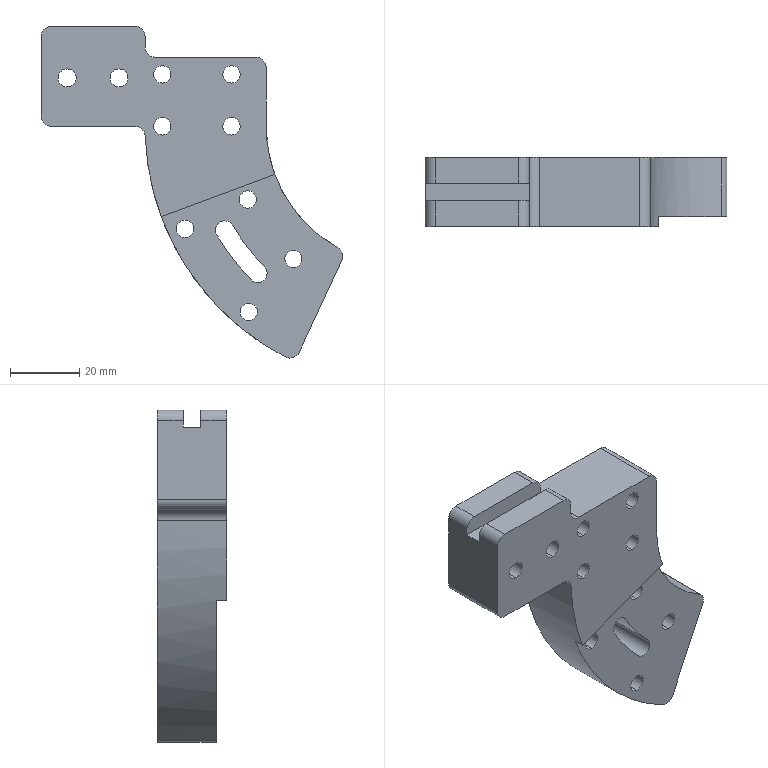Part | SolidWorks | features BaseBody 1 | 1 solid | 53 faces | box 87.153 x 20 x 95.93 mm | volume 65895 mm3 | cylinder 38 | plane 15 | commonest cylinder face diameters 5 x16 6 x11 5.2 x4 5.4 x3 80 x1 114.6 x1